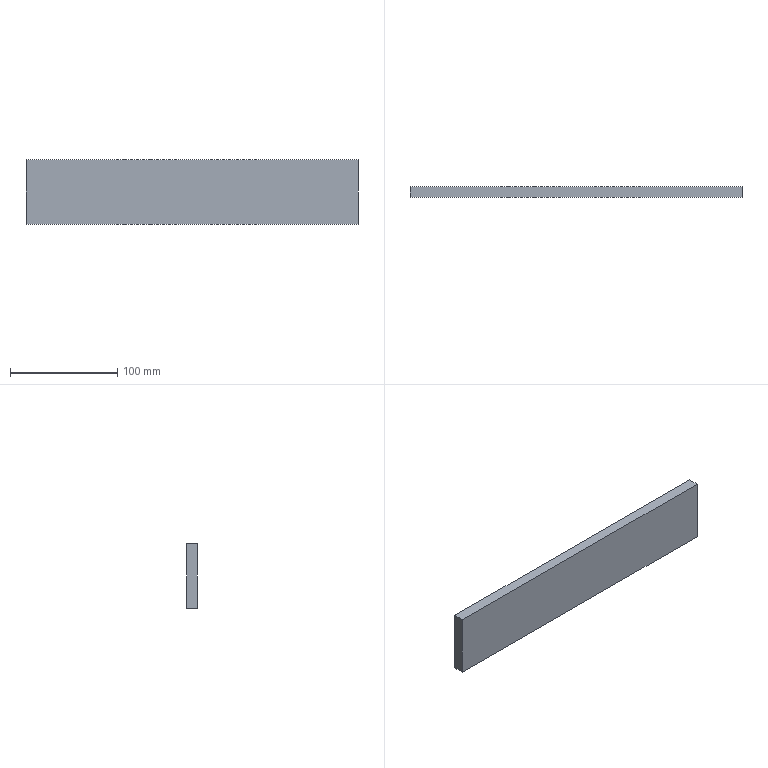Part | NX | features solid 2 | 1 solid | 6 faces | box 310 x 10 x 60 mm | volume 186000 mm3 | plane 6
STEP:
#1=CARTESIAN_POINT('',(1000.,10.,-50.));
#2=VERTEX_POINT('',#1);
#3=CARTESIAN_POINT('',(1000.,0.,-50.));
#4=VERTEX_POINT('',#3);
#5=CARTESIAN_POINT('',(1000.,10.,-50.));
#6=DIRECTION('',(0.,-1.,0.));
#7=VECTOR('',#6,1000.);
#8=LINE('',#5,#7);
#9=EDGE_CURVE('',#2,#4,#8,.T.);
#10=ORIENTED_EDGE('',*,*,#9,.T.);
#11=CARTESIAN_POINT('',(1000.,0.,-110.));
#12=VERTEX_POINT('',#11);
#13=CARTESIAN_POINT('',(1000.,0.,-50.));
#14=DIRECTION('',(0.,0.,1.));
#15=VECTOR('',#14,1000.);
#16=LINE('',#13,#15);
#17=EDGE_CURVE('',#12,#4,#16,.T.);
#18=ORIENTED_EDGE('',*,*,#17,.F.);
#19=CARTESIAN_POINT('',(1000.,10.,-110.));
#20=VERTEX_POINT('',#19);
#21=CARTESIAN_POINT('',(1000.,10.,-110.));
#22=DIRECTION('',(0.,1.,0.));
#23=VECTOR('',#22,1000.);
#24=LINE('',#21,#23);
#25=EDGE_CURVE('',#12,#20,#24,.T.);
#26=ORIENTED_EDGE('',*,*,#25,.T.);
#27=CARTESIAN_POINT('',(1000.,10.,-50.));
#28=DIRECTION('',(0.,0.,1.));
#29=VECTOR('',#28,1000.);
#30=LINE('',#27,#29);
#31=EDGE_CURVE('',#20,#2,#30,.T.);
#32=ORIENTED_EDGE('',*,*,#31,.T.);
#33=EDGE_LOOP('',(#10,#18,#26,#32));
#34=FACE_BOUND('',#33,.T.);
#35=CARTESIAN_POINT('',(1000.,10.,-50.));
#36=DIRECTION('',(-1.,0.,0.));
#37=DIRECTION('',(0.,0.,1.));
#38=AXIS2_PLACEMENT_3D('',#35,#36,#37);
#39=PLANE('',#38);
#40=ADVANCED_FACE('',(#34),#39,.F.);
#41=CARTESIAN_POINT('',(690.,10.,-50.));
#42=VERTEX_POINT('',#41);
#43=CARTESIAN_POINT('',(690.,0.,-50.));
#44=VERTEX_POINT('',#43);
#45=CARTESIAN_POINT('',(690.,0.,-50.));
#46=DIRECTION('',(0.,-1.,0.));
#47=VECTOR('',#46,1000.);
#48=LINE('',#45,#47);
#49=EDGE_CURVE('',#42,#44,#48,.T.);
#50=ORIENTED_EDGE('',*,*,#49,.T.);
#51=CARTESIAN_POINT('',(702.,0.,-50.));
#52=DIRECTION('',(-1.,0.,0.));
#53=VECTOR('',#52,1000.);
#54=LINE('',#51,#53);
#55=EDGE_CURVE('',#4,#44,#54,.T.);
#56=ORIENTED_EDGE('',*,*,#55,.F.);
#57=ORIENTED_EDGE('',*,*,#9,.F.);
#58=CARTESIAN_POINT('',(702.,10.,-50.));
#59=DIRECTION('',(-1.,0.,0.));
#60=VECTOR('',#59,1000.);
#61=LINE('',#58,#60);
#62=EDGE_CURVE('',#2,#42,#61,.T.);
#63=ORIENTED_EDGE('',*,*,#62,.T.);
#64=EDGE_LOOP('',(#50,#56,#57,#63));
#65=FACE_BOUND('',#64,.T.);
#66=CARTESIAN_POINT('',(690.,0.,-50.));
#67=DIRECTION('',(0.,0.,-1.));
#68=DIRECTION('',(-1.,0.,0.));
#69=AXIS2_PLACEMENT_3D('',#66,#67,#68);
#70=PLANE('',#69);
#71=ADVANCED_FACE('',(#65),#70,.F.);
#72=ORIENTED_EDGE('',*,*,#17,.T.);
#73=ORIENTED_EDGE('',*,*,#55,.T.);
#74=CARTESIAN_POINT('',(690.,0.,-110.));
#75=VERTEX_POINT('',#74);
#76=CARTESIAN_POINT('',(690.,0.,-120.));
#77=DIRECTION('',(0.,0.,-1.));
#78=VECTOR('',#77,1000.);
#79=LINE('',#76,#78);
#80=EDGE_CURVE('',#44,#75,#79,.T.);
#81=ORIENTED_EDGE('',*,*,#80,.T.);
#82=CARTESIAN_POINT('',(702.,0.,-110.));
#83=DIRECTION('',(1.,0.,0.));
#84=VECTOR('',#83,1000.);
#85=LINE('',#82,#84);
#86=EDGE_CURVE('',#75,#12,#85,.T.);
#87=ORIENTED_EDGE('',*,*,#86,.T.);
#88=EDGE_LOOP('',(#72,#73,#81,#87));
#89=FACE_BOUND('',#88,.T.);
#90=CARTESIAN_POINT('',(702.,0.,-120.));
#91=DIRECTION('',(0.,-1.,0.));
#92=DIRECTION('',(-1.,0.,0.));
#93=AXIS2_PLACEMENT_3D('',#90,#91,#92);
#94=PLANE('',#93);
#95=ADVANCED_FACE('',(#89),#94,.T.);
#96=ORIENTED_EDGE('',*,*,#25,.F.);
#97=ORIENTED_EDGE('',*,*,#86,.F.);
#98=CARTESIAN_POINT('',(690.,10.,-110.));
#99=VERTEX_POINT('',#98);
#100=CARTESIAN_POINT('',(690.,10.,-110.));
#101=DIRECTION('',(0.,1.,0.));
#102=VECTOR('',#101,1000.);
#103=LINE('',#100,#102);
#104=EDGE_CURVE('',#75,#99,#103,.T.);
#105=ORIENTED_EDGE('',*,*,#104,.T.);
#106=CARTESIAN_POINT('',(702.,10.,-110.));
#107=DIRECTION('',(1.,0.,0.));
#108=VECTOR('',#107,1000.);
#109=LINE('',#106,#108);
#110=EDGE_CURVE('',#99,#20,#109,.T.);
#111=ORIENTED_EDGE('',*,*,#110,.T.);
#112=EDGE_LOOP('',(#96,#97,#105,#111));
#113=FACE_BOUND('',#112,.T.);
#114=CARTESIAN_POINT('',(690.,10.,-110.));
#115=DIRECTION('',(0.,0.,1.));
#116=DIRECTION('',(0.,-1.,0.));
#117=AXIS2_PLACEMENT_3D('',#114,#115,#116);
#118=PLANE('',#117);
#119=ADVANCED_FACE('',(#113),#118,.F.);
#120=ORIENTED_EDGE('',*,*,#62,.F.);
#121=ORIENTED_EDGE('',*,*,#31,.F.);
#122=ORIENTED_EDGE('',*,*,#110,.F.);
#123=CARTESIAN_POINT('',(690.,10.,-120.));
#124=DIRECTION('',(0.,0.,1.));
#125=VECTOR('',#124,1000.);
#126=LINE('',#123,#125);
#127=EDGE_CURVE('',#99,#42,#126,.T.);
#128=ORIENTED_EDGE('',*,*,#127,.T.);
#129=EDGE_LOOP('',(#120,#121,#122,#128));
#130=FACE_BOUND('',#129,.T.);
#131=CARTESIAN_POINT('',(702.,10.,-120.));
#132=DIRECTION('',(0.,-1.,0.));
#133=DIRECTION('',(-1.,0.,0.));
#134=AXIS2_PLACEMENT_3D('',#131,#132,#133);
#135=PLANE('',#134);
#136=ADVANCED_FACE('',(#130),#135,.F.);
#137=ORIENTED_EDGE('',*,*,#104,.F.);
#138=ORIENTED_EDGE('',*,*,#80,.F.);
#139=ORIENTED_EDGE('',*,*,#49,.F.);
#140=ORIENTED_EDGE('',*,*,#127,.F.);
#141=EDGE_LOOP('',(#137,#138,#139,#140));
#142=FACE_BOUND('',#141,.T.);
#143=CARTESIAN_POINT('',(690.,10.,-120.));
#144=DIRECTION('',(1.,0.,0.));
#145=DIRECTION('',(0.,-1.,0.));
#146=AXIS2_PLACEMENT_3D('',#143,#144,#145);
#147=PLANE('',#146);
#148=ADVANCED_FACE('',(#142),#147,.F.);
#149=CLOSED_SHELL('',(#40,#71,#95,#119,#136,#148));
#150=MANIFOLD_SOLID_BREP('',#149);
#151=(LENGTH_UNIT()NAMED_UNIT(*)SI_UNIT(.MILLI.,.METRE.));
#152=UNCERTAINTY_MEASURE_WITH_UNIT(LENGTH_MEASURE(0.00001),#151,'','');
#153=(NAMED_UNIT(*)PLANE_ANGLE_UNIT()SI_UNIT($,.RADIAN.));
#154=(NAMED_UNIT(*)SI_UNIT($,.STERADIAN.)SOLID_ANGLE_UNIT());
#155=(GEOMETRIC_REPRESENTATION_CONTEXT(3)GLOBAL_UNCERTAINTY_ASSIGNED_CONTEXT((#152))GLOBAL_UNIT_ASSIGNED_CONTEXT((#151,#153,#154))REPRESENTATION_CONTEXT('',''));
#156=ADVANCED_BREP_SHAPE_REPRESENTATION('',(#150),#155);